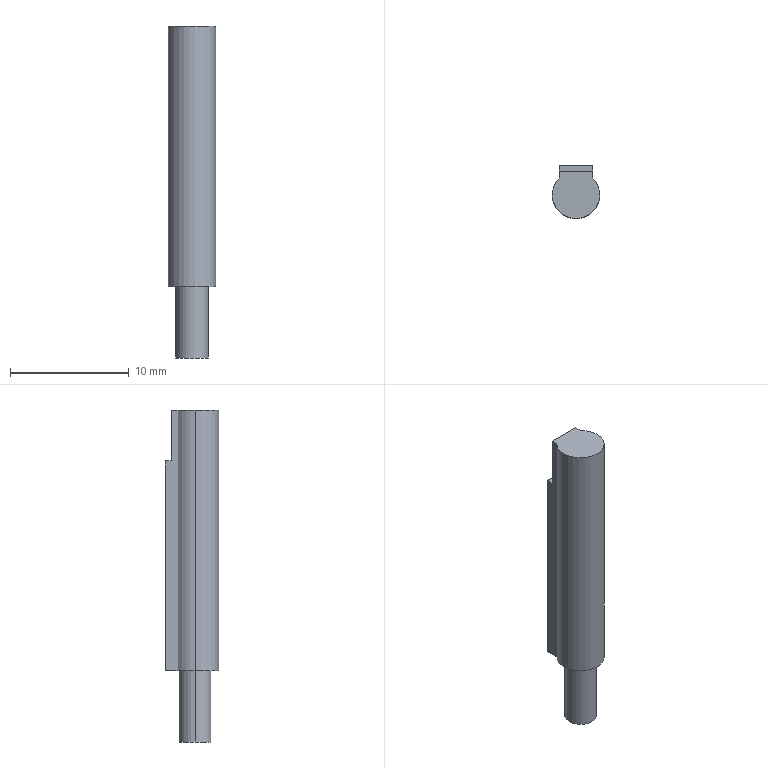Part | SolidWorks | features ICE 3, RefAxis 3, 3DProfileFeature 1, Extrusion 1 | 1 solid | 19 faces | box 4 x 4.5 x 28 mm | volume 345.122 mm3 | plane 10 | cylinder 9 | commonest cylinder face diameters 4 x3 2.1 x2 2.5 x2 2.7 x2
STEP:
#1=CARTESIAN_POINT('',(1.35,0.,-28.));
#2=VERTEX_POINT('',#1);
#3=CARTESIAN_POINT('',(-1.35,0.,-28.));
#4=VERTEX_POINT('',#3);
#5=CARTESIAN_POINT('',(0.,0.,-28.));
#6=DIRECTION('',(0.,0.,1.));
#7=DIRECTION('',(1.,0.,0.));
#8=AXIS2_PLACEMENT_3D('',#5,#6,#7);
#9=CIRCLE('',#8,1.35);
#10=EDGE_CURVE('',#2,#4,#9,.T.);
#11=ORIENTED_EDGE('',*,*,#10,.T.);
#12=CARTESIAN_POINT('',(-1.35,0.,-22.));
#13=VERTEX_POINT('',#12);
#14=CARTESIAN_POINT('',(-1.35,0.,-28.));
#15=DIRECTION('',(0.,0.,1.));
#16=VECTOR('',#15,1000.);
#17=LINE('',#14,#16);
#18=EDGE_CURVE('',#4,#13,#17,.T.);
#19=ORIENTED_EDGE('',*,*,#18,.T.);
#20=CARTESIAN_POINT('',(1.35,0.,-22.));
#21=VERTEX_POINT('',#20);
#22=CARTESIAN_POINT('',(0.,0.,-22.));
#23=DIRECTION('',(0.,0.,1.));
#24=DIRECTION('',(1.,0.,0.));
#25=AXIS2_PLACEMENT_3D('',#22,#23,#24);
#26=CIRCLE('',#25,1.35);
#27=EDGE_CURVE('',#21,#13,#26,.T.);
#28=ORIENTED_EDGE('',*,*,#27,.F.);
#29=CARTESIAN_POINT('',(1.35,0.,-28.));
#30=DIRECTION('',(0.,0.,1.));
#31=VECTOR('',#30,1000.);
#32=LINE('',#29,#31);
#33=EDGE_CURVE('',#2,#21,#32,.T.);
#34=ORIENTED_EDGE('',*,*,#33,.F.);
#35=EDGE_LOOP('',(#11,#19,#28,#34));
#36=FACE_OUTER_BOUND('',#35,.T.);
#37=CARTESIAN_POINT('',(0.,0.,-28.));
#38=DIRECTION('',(0.,0.,1.));
#39=DIRECTION('',(1.,0.,0.));
#40=AXIS2_PLACEMENT_3D('',#37,#38,#39);
#41=CYLINDRICAL_SURFACE('',#40,1.35);
#42=ADVANCED_FACE('',(#36),#41,.T.);
#43=CARTESIAN_POINT('',(0.,1.,-0.95));
#44=VERTEX_POINT('',#43);
#45=CARTESIAN_POINT('',(0.,1.,-3.05));
#46=VERTEX_POINT('',#45);
#47=CARTESIAN_POINT('',(0.,1.,-2.));
#48=DIRECTION('',(0.,1.,0.));
#49=DIRECTION('',(0.,0.,1.));
#50=AXIS2_PLACEMENT_3D('',#47,#48,#49);
#51=CIRCLE('',#50,1.05);
#52=EDGE_CURVE('',#44,#46,#51,.T.);
#53=ORIENTED_EDGE('',*,*,#52,.T.);
#54=CARTESIAN_POINT('',(0.,2.,-3.05));
#55=VERTEX_POINT('',#54);
#56=CARTESIAN_POINT('',(0.,1.,-3.05));
#57=DIRECTION('',(0.,1.,0.));
#58=VECTOR('',#57,1000.);
#59=LINE('',#56,#58);
#60=EDGE_CURVE('',#46,#55,#59,.T.);
#61=ORIENTED_EDGE('',*,*,#60,.T.);
#62=CARTESIAN_POINT('',(0.,2.,-0.95));
#63=VERTEX_POINT('',#62);
#64=CARTESIAN_POINT('',(0.,2.,-2.));
#65=DIRECTION('',(0.,1.,0.));
#66=DIRECTION('',(0.,0.,1.));
#67=AXIS2_PLACEMENT_3D('',#64,#65,#66);
#68=CIRCLE('',#67,1.05);
#69=EDGE_CURVE('',#63,#55,#68,.T.);
#70=ORIENTED_EDGE('',*,*,#69,.F.);
#71=CARTESIAN_POINT('',(0.,1.,-0.95));
#72=DIRECTION('',(0.,1.,0.));
#73=VECTOR('',#72,1000.);
#74=LINE('',#71,#73);
#75=EDGE_CURVE('',#44,#63,#74,.T.);
#76=ORIENTED_EDGE('',*,*,#75,.F.);
#77=EDGE_LOOP('',(#53,#61,#70,#76));
#78=FACE_OUTER_BOUND('',#77,.T.);
#79=CARTESIAN_POINT('',(0.,1.,-2.));
#80=DIRECTION('',(0.,1.,0.));
#81=DIRECTION('',(0.,0.,1.));
#82=AXIS2_PLACEMENT_3D('',#79,#80,#81);
#83=CYLINDRICAL_SURFACE('',#82,1.05);
#84=ADVANCED_FACE('',(#78),#83,.T.);
#85=CARTESIAN_POINT('',(0.,1.,-3.25));
#86=VERTEX_POINT('',#85);
#87=CARTESIAN_POINT('',(0.,1.,-0.75));
#88=VERTEX_POINT('',#87);
#89=CARTESIAN_POINT('',(0.,1.,-2.));
#90=DIRECTION('',(0.,1.,0.));
#91=DIRECTION('',(0.,0.,1.));
#92=AXIS2_PLACEMENT_3D('',#89,#90,#91);
#93=CIRCLE('',#92,1.25);
#94=EDGE_CURVE('',#86,#88,#93,.T.);
#95=ORIENTED_EDGE('',*,*,#94,.F.);
#96=CARTESIAN_POINT('',(0.,2.,-3.25));
#97=VERTEX_POINT('',#96);
#98=CARTESIAN_POINT('',(0.,1.,-3.25));
#99=DIRECTION('',(0.,1.,0.));
#100=VECTOR('',#99,1000.);
#101=LINE('',#98,#100);
#102=EDGE_CURVE('',#86,#97,#101,.T.);
#103=ORIENTED_EDGE('',*,*,#102,.T.);
#104=CARTESIAN_POINT('',(0.,2.,-0.75));
#105=VERTEX_POINT('',#104);
#106=CARTESIAN_POINT('',(0.,2.,-2.));
#107=DIRECTION('',(0.,1.,0.));
#108=DIRECTION('',(0.,0.,1.));
#109=AXIS2_PLACEMENT_3D('',#106,#107,#108);
#110=CIRCLE('',#109,1.25);
#111=EDGE_CURVE('',#97,#105,#110,.T.);
#112=ORIENTED_EDGE('',*,*,#111,.T.);
#113=CARTESIAN_POINT('',(0.,1.,-0.75));
#114=DIRECTION('',(0.,1.,0.));
#115=VECTOR('',#114,1000.);
#116=LINE('',#113,#115);
#117=EDGE_CURVE('',#88,#105,#116,.T.);
#118=ORIENTED_EDGE('',*,*,#117,.F.);
#119=EDGE_LOOP('',(#95,#103,#112,#118));
#120=FACE_OUTER_BOUND('',#119,.T.);
#121=CARTESIAN_POINT('',(0.,1.,-2.));
#122=DIRECTION('',(0.,1.,0.));
#123=DIRECTION('',(0.,0.,1.));
#124=AXIS2_PLACEMENT_3D('',#121,#122,#123);
#125=CYLINDRICAL_SURFACE('',#124,1.25);
#126=ADVANCED_FACE('',(#120),#125,.F.);
#127=CARTESIAN_POINT('',(-1.4,1.428,-22.));
#128=VERTEX_POINT('',#127);
#129=CARTESIAN_POINT('',(-2.,0.,-22.));
#130=VERTEX_POINT('',#129);
#131=CARTESIAN_POINT('',(0.,0.,-22.));
#132=DIRECTION('',(0.,0.,1.));
#133=DIRECTION('',(1.,0.,0.));
#134=AXIS2_PLACEMENT_3D('',#131,#132,#133);
#135=CIRCLE('',#134,2.);
#136=EDGE_CURVE('',#128,#130,#135,.T.);
#137=ORIENTED_EDGE('',*,*,#136,.T.);
#138=CARTESIAN_POINT('',(-2.,0.,0.));
#139=VERTEX_POINT('',#138);
#140=CARTESIAN_POINT('',(-2.,0.,-22.));
#141=DIRECTION('',(0.,0.,1.));
#142=VECTOR('',#141,1000.);
#143=LINE('',#140,#142);
#144=EDGE_CURVE('',#130,#139,#143,.T.);
#145=ORIENTED_EDGE('',*,*,#144,.T.);
#146=CARTESIAN_POINT('',(-1.4,1.428,0.));
#147=VERTEX_POINT('',#146);
#148=CARTESIAN_POINT('',(0.,0.,0.));
#149=DIRECTION('',(0.,0.,1.));
#150=DIRECTION('',(1.,0.,0.));
#151=AXIS2_PLACEMENT_3D('',#148,#149,#150);
#152=CIRCLE('',#151,2.);
#153=EDGE_CURVE('',#147,#139,#152,.T.);
#154=ORIENTED_EDGE('',*,*,#153,.F.);
#155=CARTESIAN_POINT('',(-1.4,1.428,-22.));
#156=DIRECTION('',(0.,0.,1.));
#157=VECTOR('',#156,1000.);
#158=LINE('',#155,#157);
#159=EDGE_CURVE('',#128,#147,#158,.T.);
#160=ORIENTED_EDGE('',*,*,#159,.F.);
#161=EDGE_LOOP('',(#137,#145,#154,#160));
#162=FACE_OUTER_BOUND('',#161,.T.);
#163=CARTESIAN_POINT('',(0.,0.,-22.));
#164=DIRECTION('',(0.,0.,1.));
#165=DIRECTION('',(1.,0.,0.));
#166=AXIS2_PLACEMENT_3D('',#163,#164,#165);
#167=CYLINDRICAL_SURFACE('',#166,2.);
#168=ADVANCED_FACE('',(#162),#167,.T.);
#169=ORIENTED_EDGE('',*,*,#144,.F.);
#170=CARTESIAN_POINT('',(2.,0.,-22.));
#171=VERTEX_POINT('',#170);
#172=CARTESIAN_POINT('',(0.,0.,-22.));
#173=DIRECTION('',(0.,0.,1.));
#174=DIRECTION('',(1.,0.,0.));
#175=AXIS2_PLACEMENT_3D('',#172,#173,#174);
#176=CIRCLE('',#175,2.);
#177=EDGE_CURVE('',#130,#171,#176,.T.);
#178=ORIENTED_EDGE('',*,*,#177,.T.);
#179=CARTESIAN_POINT('',(2.,0.,0.));
#180=VERTEX_POINT('',#179);
#181=CARTESIAN_POINT('',(2.,0.,-22.));
#182=DIRECTION('',(0.,0.,1.));
#183=VECTOR('',#182,1000.);
#184=LINE('',#181,#183);
#185=EDGE_CURVE('',#171,#180,#184,.T.);
#186=ORIENTED_EDGE('',*,*,#185,.T.);
#187=CARTESIAN_POINT('',(0.,0.,0.));
#188=DIRECTION('',(0.,0.,1.));
#189=DIRECTION('',(1.,0.,0.));
#190=AXIS2_PLACEMENT_3D('',#187,#188,#189);
#191=CIRCLE('',#190,2.);
#192=EDGE_CURVE('',#139,#180,#191,.T.);
#193=ORIENTED_EDGE('',*,*,#192,.F.);
#194=EDGE_LOOP('',(#169,#178,#186,#193));
#195=FACE_OUTER_BOUND('',#194,.T.);
#196=CARTESIAN_POINT('',(0.,0.,-22.));
#197=DIRECTION('',(0.,0.,1.));
#198=DIRECTION('',(1.,0.,0.));
#199=AXIS2_PLACEMENT_3D('',#196,#197,#198);
#200=CYLINDRICAL_SURFACE('',#199,2.);
#201=ADVANCED_FACE('',(#195),#200,.T.);
#202=ORIENTED_EDGE('',*,*,#185,.F.);
#203=CARTESIAN_POINT('',(1.4,1.428,-22.));
#204=VERTEX_POINT('',#203);
#205=CARTESIAN_POINT('',(0.,0.,-22.));
#206=DIRECTION('',(0.,0.,1.));
#207=DIRECTION('',(1.,0.,0.));
#208=AXIS2_PLACEMENT_3D('',#205,#206,#207);
#209=CIRCLE('',#208,2.);
#210=EDGE_CURVE('',#171,#204,#209,.T.);
#211=ORIENTED_EDGE('',*,*,#210,.T.);
#212=CARTESIAN_POINT('',(1.4,1.428,0.));
#213=VERTEX_POINT('',#212);
#214=CARTESIAN_POINT('',(1.4,1.428,-22.));
#215=DIRECTION('',(0.,0.,1.));
#216=VECTOR('',#215,1000.);
#217=LINE('',#214,#216);
#218=EDGE_CURVE('',#204,#213,#217,.T.);
#219=ORIENTED_EDGE('',*,*,#218,.T.);
#220=CARTESIAN_POINT('',(0.,0.,0.));
#221=DIRECTION('',(0.,0.,1.));
#222=DIRECTION('',(1.,0.,0.));
#223=AXIS2_PLACEMENT_3D('',#220,#221,#222);
#224=CIRCLE('',#223,2.);
#225=EDGE_CURVE('',#180,#213,#224,.T.);
#226=ORIENTED_EDGE('',*,*,#225,.F.);
#227=EDGE_LOOP('',(#202,#211,#219,#226));
#228=FACE_OUTER_BOUND('',#227,.T.);
#229=CARTESIAN_POINT('',(0.,0.,-22.));
#230=DIRECTION('',(0.,0.,1.));
#231=DIRECTION('',(1.,0.,0.));
#232=AXIS2_PLACEMENT_3D('',#229,#230,#231);
#233=CYLINDRICAL_SURFACE('',#232,2.);
#234=ADVANCED_FACE('',(#228),#233,.T.);
#235=CARTESIAN_POINT('',(-1.4,2.,0.));
#236=VERTEX_POINT('',#235);
#237=CARTESIAN_POINT('',(-1.4,2.,0.));
#238=DIRECTION('',(0.,-1.,0.));
#239=VECTOR('',#238,1000.);
#240=LINE('',#237,#239);
#241=EDGE_CURVE('',#236,#147,#240,.T.);
#242=ORIENTED_EDGE('',*,*,#241,.F.);
#243=CARTESIAN_POINT('',(-1.4,2.,-4.3));
#244=VERTEX_POINT('',#243);
#245=CARTESIAN_POINT('',(-1.4,2.,-22.));
#246=DIRECTION('',(0.,0.,1.));
#247=VECTOR('',#246,1000.);
#248=LINE('',#245,#247);
#249=EDGE_CURVE('',#244,#236,#248,.T.);
#250=ORIENTED_EDGE('',*,*,#249,.F.);
#251=CARTESIAN_POINT('',(-1.4,2.5,-4.3));
#252=VERTEX_POINT('',#251);
#253=CARTESIAN_POINT('',(-1.4,2.5,-4.3));
#254=DIRECTION('',(0.,-1.,0.));
#255=VECTOR('',#254,1000.);
#256=LINE('',#253,#255);
#257=EDGE_CURVE('',#252,#244,#256,.T.);
#258=ORIENTED_EDGE('',*,*,#257,.F.);
#259=CARTESIAN_POINT('',(-1.4,2.5,-22.));
#260=VERTEX_POINT('',#259);
#261=CARTESIAN_POINT('',(-1.4,2.5,-4.3));
#262=DIRECTION('',(0.,0.,-1.));
#263=VECTOR('',#262,1000.);
#264=LINE('',#261,#263);
#265=EDGE_CURVE('',#252,#260,#264,.T.);
#266=ORIENTED_EDGE('',*,*,#265,.T.);
#267=CARTESIAN_POINT('',(-1.4,2.,-22.));
#268=DIRECTION('',(0.,-1.,0.));
#269=VECTOR('',#268,1000.);
#270=LINE('',#267,#269);
#271=EDGE_CURVE('',#260,#128,#270,.T.);
#272=ORIENTED_EDGE('',*,*,#271,.T.);
#273=ORIENTED_EDGE('',*,*,#159,.T.);
#274=EDGE_LOOP('',(#242,#250,#258,#266,#272,#273));
#275=FACE_OUTER_BOUND('',#274,.T.);
#276=CARTESIAN_POINT('',(-1.4,2.,-22.));
#277=DIRECTION('',(-1.,0.,0.));
#278=DIRECTION('',(0.,0.,1.));
#279=AXIS2_PLACEMENT_3D('',#276,#277,#278);
#280=PLANE('',#279);
#281=ADVANCED_FACE('',(#275),#280,.T.);
#282=CARTESIAN_POINT('',(0.,2.,-2.));
#283=DIRECTION('',(0.,1.,0.));
#284=DIRECTION('',(0.,0.,1.));
#285=AXIS2_PLACEMENT_3D('',#282,#283,#284);
#286=CIRCLE('',#285,1.25);
#287=EDGE_CURVE('',#105,#97,#286,.T.);
#288=ORIENTED_EDGE('',*,*,#287,.F.);
#289=ORIENTED_EDGE('',*,*,#111,.F.);
#290=EDGE_LOOP('',(#288,#289));
#291=FACE_BOUND('',#290,.T.);
#292=CARTESIAN_POINT('',(1.4,2.,-4.3));
#293=VERTEX_POINT('',#292);
#294=CARTESIAN_POINT('',(-1.4,2.,-4.3));
#295=DIRECTION('',(1.,0.,0.));
#296=VECTOR('',#295,1000.);
#297=LINE('',#294,#296);
#298=EDGE_CURVE('',#244,#293,#297,.T.);
#299=ORIENTED_EDGE('',*,*,#298,.F.);
#300=ORIENTED_EDGE('',*,*,#249,.T.);
#301=CARTESIAN_POINT('',(1.4,2.,0.));
#302=VERTEX_POINT('',#301);
#303=CARTESIAN_POINT('',(1.4,2.,0.));
#304=DIRECTION('',(-1.,0.,0.));
#305=VECTOR('',#304,1000.);
#306=LINE('',#303,#305);
#307=EDGE_CURVE('',#302,#236,#306,.T.);
#308=ORIENTED_EDGE('',*,*,#307,.F.);
#309=CARTESIAN_POINT('',(1.4,2.,-22.));
#310=DIRECTION('',(0.,0.,1.));
#311=VECTOR('',#310,1000.);
#312=LINE('',#309,#311);
#313=EDGE_CURVE('',#293,#302,#312,.T.);
#314=ORIENTED_EDGE('',*,*,#313,.F.);
#315=EDGE_LOOP('',(#299,#300,#308,#314));
#316=FACE_OUTER_BOUND('',#315,.T.);
#317=CARTESIAN_POINT('',(1.4,2.,-22.));
#318=DIRECTION('',(0.,1.,0.));
#319=DIRECTION('',(-1.,0.,0.));
#320=AXIS2_PLACEMENT_3D('',#317,#318,#319);
#321=PLANE('',#320);
#322=ADVANCED_FACE('',(#291,#316),#321,.T.);
#323=CARTESIAN_POINT('',(1.4,1.428,0.));
#324=DIRECTION('',(0.,1.,0.));
#325=VECTOR('',#324,1000.);
#326=LINE('',#323,#325);
#327=EDGE_CURVE('',#213,#302,#326,.T.);
#328=ORIENTED_EDGE('',*,*,#327,.F.);
#329=ORIENTED_EDGE('',*,*,#218,.F.);
#330=CARTESIAN_POINT('',(1.4,2.5,-22.));
#331=VERTEX_POINT('',#330);
#332=CARTESIAN_POINT('',(1.4,1.428,-22.));
#333=DIRECTION('',(0.,1.,0.));
#334=VECTOR('',#333,1000.);
#335=LINE('',#332,#334);
#336=EDGE_CURVE('',#204,#331,#335,.T.);
#337=ORIENTED_EDGE('',*,*,#336,.T.);
#338=CARTESIAN_POINT('',(1.4,2.5,-4.3));
#339=VERTEX_POINT('',#338);
#340=CARTESIAN_POINT('',(1.4,2.5,-4.3));
#341=DIRECTION('',(0.,0.,-1.));
#342=VECTOR('',#341,1000.);
#343=LINE('',#340,#342);
#344=EDGE_CURVE('',#339,#331,#343,.T.);
#345=ORIENTED_EDGE('',*,*,#344,.F.);
#346=CARTESIAN_POINT('',(1.4,2.,-4.3));
#347=DIRECTION('',(0.,1.,0.));
#348=VECTOR('',#347,1000.);
#349=LINE('',#346,#348);
#350=EDGE_CURVE('',#293,#339,#349,.T.);
#351=ORIENTED_EDGE('',*,*,#350,.F.);
#352=ORIENTED_EDGE('',*,*,#313,.T.);
#353=EDGE_LOOP('',(#328,#329,#337,#345,#351,#352));
#354=FACE_OUTER_BOUND('',#353,.T.);
#355=CARTESIAN_POINT('',(1.4,1.428,-22.));
#356=DIRECTION('',(1.,0.,0.));
#357=DIRECTION('',(0.,0.,-1.));
#358=AXIS2_PLACEMENT_3D('',#355,#356,#357);
#359=PLANE('',#358);
#360=ADVANCED_FACE('',(#354),#359,.T.);
#361=ORIENTED_EDGE('',*,*,#27,.T.);
#362=CARTESIAN_POINT('',(0.,0.,-22.));
#363=DIRECTION('',(0.,0.,1.));
#364=DIRECTION('',(1.,0.,0.));
#365=AXIS2_PLACEMENT_3D('',#362,#363,#364);
#366=CIRCLE('',#365,1.35);
#367=EDGE_CURVE('',#13,#21,#366,.T.);
#368=ORIENTED_EDGE('',*,*,#367,.T.);
#369=EDGE_LOOP('',(#361,#368));
#370=FACE_BOUND('',#369,.T.);
#371=ORIENTED_EDGE('',*,*,#136,.F.);
#372=ORIENTED_EDGE('',*,*,#271,.F.);
#373=CARTESIAN_POINT('',(1.4,2.5,-22.));
#374=DIRECTION('',(-1.,0.,0.));
#375=VECTOR('',#374,1000.);
#376=LINE('',#373,#375);
#377=EDGE_CURVE('',#331,#260,#376,.T.);
#378=ORIENTED_EDGE('',*,*,#377,.F.);
#379=ORIENTED_EDGE('',*,*,#336,.F.);
#380=ORIENTED_EDGE('',*,*,#210,.F.);
#381=ORIENTED_EDGE('',*,*,#177,.F.);
#382=EDGE_LOOP('',(#371,#372,#378,#379,#380,#381));
#383=FACE_OUTER_BOUND('',#382,.T.);
#384=CARTESIAN_POINT('',(0.,0.,-22.));
#385=DIRECTION('',(0.,0.,1.));
#386=DIRECTION('',(1.,0.,0.));
#387=AXIS2_PLACEMENT_3D('',#384,#385,#386);
#388=PLANE('',#387);
#389=ADVANCED_FACE('',(#370,#383),#388,.F.);
#390=ORIENTED_EDGE('',*,*,#153,.T.);
#391=ORIENTED_EDGE('',*,*,#192,.T.);
#392=ORIENTED_EDGE('',*,*,#225,.T.);
#393=ORIENTED_EDGE('',*,*,#327,.T.);
#394=ORIENTED_EDGE('',*,*,#307,.T.);
#395=ORIENTED_EDGE('',*,*,#241,.T.);
#396=EDGE_LOOP('',(#390,#391,#392,#393,#394,#395));
#397=FACE_OUTER_BOUND('',#396,.T.);
#398=CARTESIAN_POINT('',(0.,0.,0.));
#399=DIRECTION('',(0.,0.,1.));
#400=DIRECTION('',(1.,0.,0.));
#401=AXIS2_PLACEMENT_3D('',#398,#399,#400);
#402=PLANE('',#401);
#403=ADVANCED_FACE('',(#397),#402,.T.);
#404=ORIENTED_EDGE('',*,*,#377,.T.);
#405=ORIENTED_EDGE('',*,*,#265,.F.);
#406=CARTESIAN_POINT('',(1.4,2.5,-4.3));
#407=DIRECTION('',(-1.,0.,0.));
#408=VECTOR('',#407,1000.);
#409=LINE('',#406,#408);
#410=EDGE_CURVE('',#339,#252,#409,.T.);
#411=ORIENTED_EDGE('',*,*,#410,.F.);
#412=ORIENTED_EDGE('',*,*,#344,.T.);
#413=EDGE_LOOP('',(#404,#405,#411,#412));
#414=FACE_OUTER_BOUND('',#413,.T.);
#415=CARTESIAN_POINT('',(1.4,2.5,-4.3));
#416=DIRECTION('',(0.,-1.,0.));
#417=DIRECTION('',(0.,0.,-1.));
#418=AXIS2_PLACEMENT_3D('',#415,#416,#417);
#419=PLANE('',#418);
#420=ADVANCED_FACE('',(#414),#419,.F.);
#421=ORIENTED_EDGE('',*,*,#410,.T.);
#422=ORIENTED_EDGE('',*,*,#257,.T.);
#423=ORIENTED_EDGE('',*,*,#298,.T.);
#424=ORIENTED_EDGE('',*,*,#350,.T.);
#425=EDGE_LOOP('',(#421,#422,#423,#424));
#426=FACE_OUTER_BOUND('',#425,.T.);
#427=CARTESIAN_POINT('',(0.,0.,-4.3));
#428=DIRECTION('',(0.,0.,1.));
#429=DIRECTION('',(1.,0.,0.));
#430=AXIS2_PLACEMENT_3D('',#427,#428,#429);
#431=PLANE('',#430);
#432=ADVANCED_FACE('',(#426),#431,.T.);
#433=ORIENTED_EDGE('',*,*,#102,.F.);
#434=CARTESIAN_POINT('',(0.,1.,-2.));
#435=DIRECTION('',(0.,1.,0.));
#436=DIRECTION('',(0.,0.,1.));
#437=AXIS2_PLACEMENT_3D('',#434,#435,#436);
#438=CIRCLE('',#437,1.25);
#439=EDGE_CURVE('',#88,#86,#438,.T.);
#440=ORIENTED_EDGE('',*,*,#439,.F.);
#441=ORIENTED_EDGE('',*,*,#117,.T.);
#442=ORIENTED_EDGE('',*,*,#287,.T.);
#443=EDGE_LOOP('',(#433,#440,#441,#442));
#444=FACE_OUTER_BOUND('',#443,.T.);
#445=CARTESIAN_POINT('',(0.,1.,-2.));
#446=DIRECTION('',(0.,1.,0.));
#447=DIRECTION('',(0.,0.,1.));
#448=AXIS2_PLACEMENT_3D('',#445,#446,#447);
#449=CYLINDRICAL_SURFACE('',#448,1.25);
#450=ADVANCED_FACE('',(#444),#449,.F.);
#451=ORIENTED_EDGE('',*,*,#52,.F.);
#452=CARTESIAN_POINT('',(0.,1.,-2.));
#453=DIRECTION('',(0.,1.,0.));
#454=DIRECTION('',(0.,0.,1.));
#455=AXIS2_PLACEMENT_3D('',#452,#453,#454);
#456=CIRCLE('',#455,1.05);
#457=EDGE_CURVE('',#46,#44,#456,.T.);
#458=ORIENTED_EDGE('',*,*,#457,.F.);
#459=EDGE_LOOP('',(#451,#458));
#460=FACE_BOUND('',#459,.T.);
#461=ORIENTED_EDGE('',*,*,#439,.T.);
#462=ORIENTED_EDGE('',*,*,#94,.T.);
#463=EDGE_LOOP('',(#461,#462));
#464=FACE_OUTER_BOUND('',#463,.T.);
#465=CARTESIAN_POINT('',(0.,1.,-2.));
#466=DIRECTION('',(0.,1.,0.));
#467=DIRECTION('',(0.,0.,1.));
#468=AXIS2_PLACEMENT_3D('',#465,#466,#467);
#469=PLANE('',#468);
#470=ADVANCED_FACE('',(#460,#464),#469,.T.);
#471=ORIENTED_EDGE('',*,*,#60,.F.);
#472=ORIENTED_EDGE('',*,*,#457,.T.);
#473=ORIENTED_EDGE('',*,*,#75,.T.);
#474=CARTESIAN_POINT('',(0.,2.,-2.));
#475=DIRECTION('',(0.,1.,0.));
#476=DIRECTION('',(0.,0.,1.));
#477=AXIS2_PLACEMENT_3D('',#474,#475,#476);
#478=CIRCLE('',#477,1.05);
#479=EDGE_CURVE('',#55,#63,#478,.T.);
#480=ORIENTED_EDGE('',*,*,#479,.F.);
#481=EDGE_LOOP('',(#471,#472,#473,#480));
#482=FACE_OUTER_BOUND('',#481,.T.);
#483=CARTESIAN_POINT('',(0.,1.,-2.));
#484=DIRECTION('',(0.,1.,0.));
#485=DIRECTION('',(0.,0.,1.));
#486=AXIS2_PLACEMENT_3D('',#483,#484,#485);
#487=CYLINDRICAL_SURFACE('',#486,1.05);
#488=ADVANCED_FACE('',(#482),#487,.T.);
#489=ORIENTED_EDGE('',*,*,#69,.T.);
#490=ORIENTED_EDGE('',*,*,#479,.T.);
#491=EDGE_LOOP('',(#489,#490));
#492=FACE_OUTER_BOUND('',#491,.T.);
#493=CARTESIAN_POINT('',(1.4,2.,-22.));
#494=DIRECTION('',(0.,1.,0.));
#495=DIRECTION('',(-1.,0.,0.));
#496=AXIS2_PLACEMENT_3D('',#493,#494,#495);
#497=PLANE('',#496);
#498=ADVANCED_FACE('',(#492),#497,.T.);
#499=ORIENTED_EDGE('',*,*,#18,.F.);
#500=CARTESIAN_POINT('',(0.,0.,-28.));
#501=DIRECTION('',(0.,0.,1.));
#502=DIRECTION('',(1.,0.,0.));
#503=AXIS2_PLACEMENT_3D('',#500,#501,#502);
#504=CIRCLE('',#503,1.35);
#505=EDGE_CURVE('',#4,#2,#504,.T.);
#506=ORIENTED_EDGE('',*,*,#505,.T.);
#507=ORIENTED_EDGE('',*,*,#33,.T.);
#508=ORIENTED_EDGE('',*,*,#367,.F.);
#509=EDGE_LOOP('',(#499,#506,#507,#508));
#510=FACE_OUTER_BOUND('',#509,.T.);
#511=CARTESIAN_POINT('',(0.,0.,-28.));
#512=DIRECTION('',(0.,0.,1.));
#513=DIRECTION('',(1.,0.,0.));
#514=AXIS2_PLACEMENT_3D('',#511,#512,#513);
#515=CYLINDRICAL_SURFACE('',#514,1.35);
#516=ADVANCED_FACE('',(#510),#515,.T.);
#517=ORIENTED_EDGE('',*,*,#10,.F.);
#518=ORIENTED_EDGE('',*,*,#505,.F.);
#519=EDGE_LOOP('',(#517,#518));
#520=FACE_OUTER_BOUND('',#519,.T.);
#521=CARTESIAN_POINT('',(0.,0.,-28.));
#522=DIRECTION('',(0.,0.,1.));
#523=DIRECTION('',(1.,0.,0.));
#524=AXIS2_PLACEMENT_3D('',#521,#522,#523);
#525=PLANE('',#524);
#526=ADVANCED_FACE('',(#520),#525,.F.);
#527=CLOSED_SHELL('',(#42,#84,#126,#168,#201,#234,#281,#322,#360,#389,#403,#420,#432,#450,#470,#488,#498,#516,#526));
#528=MANIFOLD_SOLID_BREP('',#527);
#529=CARTESIAN_POINT('',(0.,0.,0.));
#530=DIRECTION('',(0.,0.,1.));
#531=DIRECTION('',(1.,0.,0.));
#532=AXIS2_PLACEMENT_3D('',#529,#530,#531);
#533=(LENGTH_UNIT()NAMED_UNIT(*)SI_UNIT(.MILLI.,.METRE.));
#534=UNCERTAINTY_MEASURE_WITH_UNIT(LENGTH_MEASURE(0.00001),#533,'','');
#535=(NAMED_UNIT(*)PLANE_ANGLE_UNIT()SI_UNIT($,.RADIAN.));
#536=(NAMED_UNIT(*)SI_UNIT($,.STERADIAN.)SOLID_ANGLE_UNIT());
#537=(GEOMETRIC_REPRESENTATION_CONTEXT(3)GLOBAL_UNCERTAINTY_ASSIGNED_CONTEXT((#534))GLOBAL_UNIT_ASSIGNED_CONTEXT((#533,#535,#536))REPRESENTATION_CONTEXT('',''));
#538=ADVANCED_BREP_SHAPE_REPRESENTATION('',(#528,#532),#537);